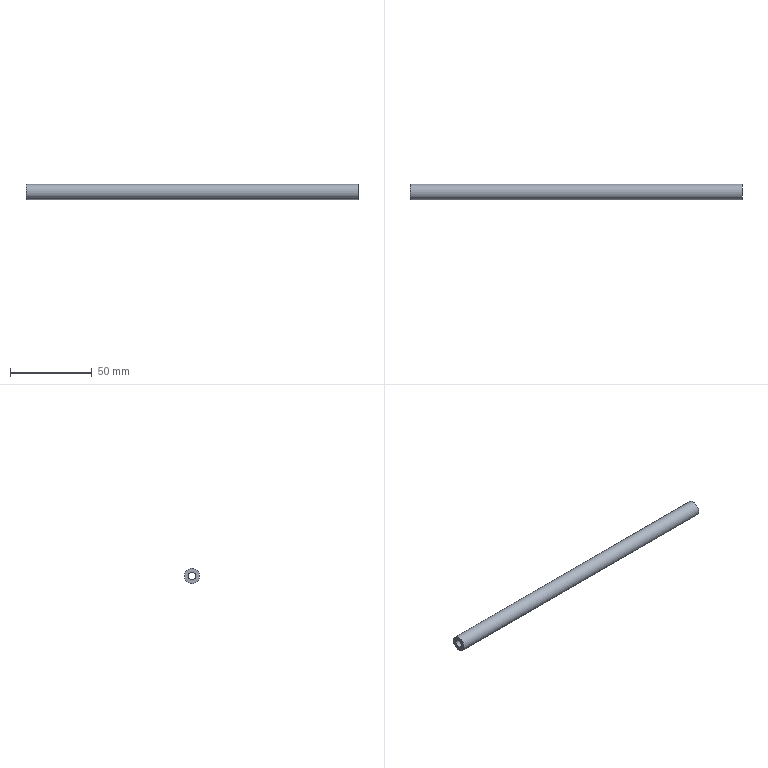Part | NX | features MG0316 door pushrod 2 | 1 solid | 4 faces | box 203.2 x 9.335 x 9.335 mm | volume 10286 mm3 | plane 2 | cylinder 2 | commonest cylinder face diameters 4.763 x1 9.335 x1
STEP:
#1=CARTESIAN_POINT('',(19.05,0.,2.381));
#2=VERTEX_POINT('',#1);
#3=CARTESIAN_POINT('',(19.05,0.,0.));
#4=DIRECTION('',(-1.,0.,0.));
#5=DIRECTION('',(0.,0.,1.));
#6=AXIS2_PLACEMENT_3D('',#3,#4,#5);
#7=CIRCLE('',#6,2.381);
#8=EDGE_CURVE('',#2,#2,#7,.T.);
#9=ORIENTED_EDGE('',*,*,#8,.F.);
#10=EDGE_LOOP('',(#9));
#11=FACE_BOUND('',#10,.T.);
#12=CARTESIAN_POINT('',(19.05,0.,4.667));
#13=VERTEX_POINT('',#12);
#14=CARTESIAN_POINT('',(19.05,0.,0.));
#15=DIRECTION('',(-1.,0.,0.));
#16=DIRECTION('',(0.,0.,1.));
#17=AXIS2_PLACEMENT_3D('',#14,#15,#16);
#18=CIRCLE('',#17,4.667);
#19=EDGE_CURVE('',#13,#13,#18,.T.);
#20=ORIENTED_EDGE('',*,*,#19,.T.);
#21=EDGE_LOOP('',(#20));
#22=FACE_BOUND('',#21,.T.);
#23=CARTESIAN_POINT('',(19.05,4.667,0.));
#24=DIRECTION('',(1.,0.,0.));
#25=DIRECTION('',(0.,0.,-1.));
#26=AXIS2_PLACEMENT_3D('',#23,#24,#25);
#27=PLANE('',#26);
#28=ADVANCED_FACE('',(#11,#22),#27,.F.);
#29=CARTESIAN_POINT('',(222.25,0.,2.381));
#30=VERTEX_POINT('',#29);
#31=CARTESIAN_POINT('',(222.25,0.,0.));
#32=DIRECTION('',(-1.,0.,0.));
#33=DIRECTION('',(0.,0.,1.));
#34=AXIS2_PLACEMENT_3D('',#31,#32,#33);
#35=CIRCLE('',#34,2.381);
#36=EDGE_CURVE('',#30,#30,#35,.T.);
#37=ORIENTED_EDGE('',*,*,#36,.F.);
#38=EDGE_LOOP('',(#37));
#39=FACE_BOUND('',#38,.T.);
#40=ORIENTED_EDGE('',*,*,#8,.T.);
#41=EDGE_LOOP('',(#40));
#42=FACE_BOUND('',#41,.T.);
#43=CARTESIAN_POINT('',(0.,0.,0.));
#44=DIRECTION('',(-1.,0.,0.));
#45=DIRECTION('',(0.,0.,1.));
#46=AXIS2_PLACEMENT_3D('',#43,#44,#45);
#47=CYLINDRICAL_SURFACE('',#46,2.381);
#48=ADVANCED_FACE('',(#39,#42),#47,.F.);
#49=CARTESIAN_POINT('',(222.25,0.,4.667));
#50=VERTEX_POINT('',#49);
#51=CARTESIAN_POINT('',(222.25,0.,0.));
#52=DIRECTION('',(-1.,0.,0.));
#53=DIRECTION('',(0.,0.,1.));
#54=AXIS2_PLACEMENT_3D('',#51,#52,#53);
#55=CIRCLE('',#54,4.667);
#56=EDGE_CURVE('',#50,#50,#55,.T.);
#57=ORIENTED_EDGE('',*,*,#56,.F.);
#58=EDGE_LOOP('',(#57));
#59=FACE_BOUND('',#58,.T.);
#60=ORIENTED_EDGE('',*,*,#36,.T.);
#61=EDGE_LOOP('',(#60));
#62=FACE_BOUND('',#61,.T.);
#63=CARTESIAN_POINT('',(222.25,4.667,0.));
#64=DIRECTION('',(-1.,0.,0.));
#65=DIRECTION('',(0.,0.,1.));
#66=AXIS2_PLACEMENT_3D('',#63,#64,#65);
#67=PLANE('',#66);
#68=ADVANCED_FACE('',(#59,#62),#67,.F.);
#69=ORIENTED_EDGE('',*,*,#19,.F.);
#70=EDGE_LOOP('',(#69));
#71=FACE_BOUND('',#70,.T.);
#72=ORIENTED_EDGE('',*,*,#56,.T.);
#73=EDGE_LOOP('',(#72));
#74=FACE_BOUND('',#73,.T.);
#75=CARTESIAN_POINT('',(0.,0.,0.));
#76=DIRECTION('',(-1.,0.,0.));
#77=DIRECTION('',(0.,0.,1.));
#78=AXIS2_PLACEMENT_3D('',#75,#76,#77);
#79=CYLINDRICAL_SURFACE('',#78,4.667);
#80=ADVANCED_FACE('',(#71,#74),#79,.T.);
#81=CLOSED_SHELL('',(#28,#48,#68,#80));
#82=MANIFOLD_SOLID_BREP('',#81);
#83=(LENGTH_UNIT()NAMED_UNIT(*)SI_UNIT(.MILLI.,.METRE.));
#84=UNCERTAINTY_MEASURE_WITH_UNIT(LENGTH_MEASURE(0.00001),#83,'','');
#85=(NAMED_UNIT(*)PLANE_ANGLE_UNIT()SI_UNIT($,.RADIAN.));
#86=(NAMED_UNIT(*)SI_UNIT($,.STERADIAN.)SOLID_ANGLE_UNIT());
#87=(GEOMETRIC_REPRESENTATION_CONTEXT(3)GLOBAL_UNCERTAINTY_ASSIGNED_CONTEXT((#84))GLOBAL_UNIT_ASSIGNED_CONTEXT((#83,#85,#86))REPRESENTATION_CONTEXT('',''));
#88=ADVANCED_BREP_SHAPE_REPRESENTATION('',(#82),#87);